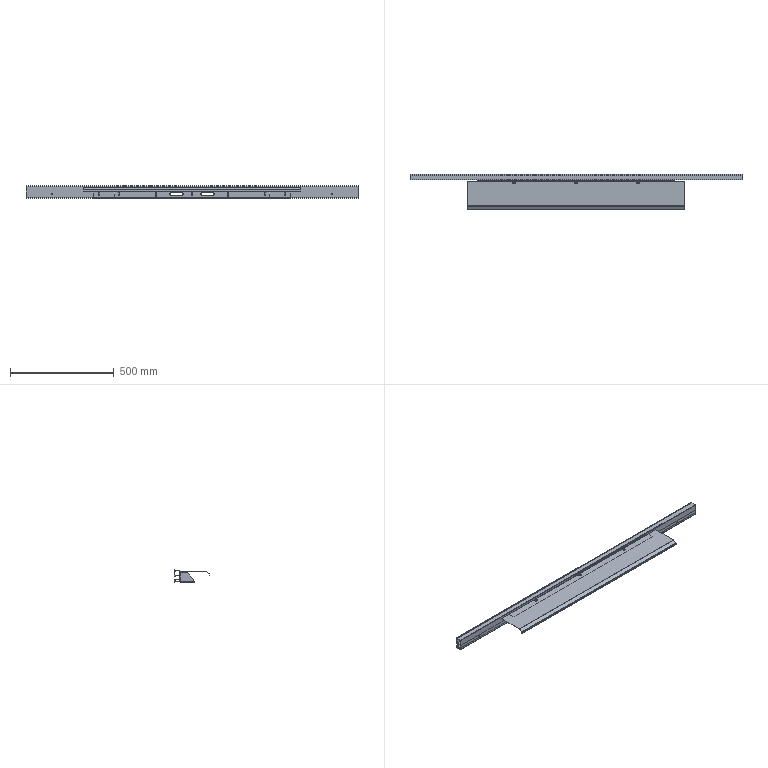Part | 8 solids | 267 faces | box 1600 x 170.821 x 60 mm | volume 1206888 mm3 | plane 153 | cylinder 114 | commonest cylinder face diameters 7 x43 6 x15 2 x13 11 x12 1 x6 10 x6